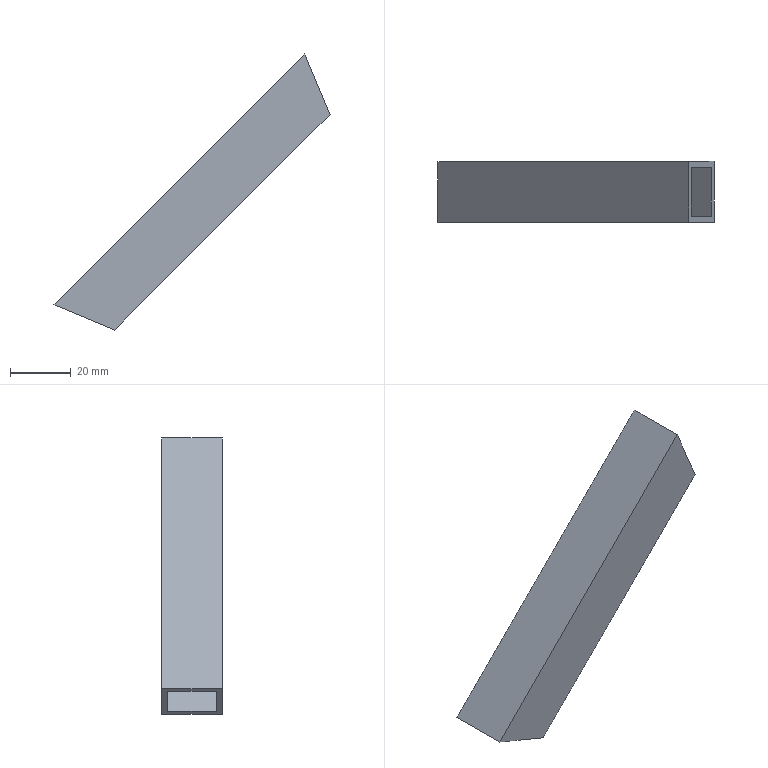Part | NX | features BREP 1 | 1 solid | 10 faces | box 90.584 x 20 x 90.584 mm | volume 15567 mm3 | plane 10
STEP:
#1=CARTESIAN_POINT('',(759.673,696.,1230.563));
#2=VERTEX_POINT('',#1);
#3=CARTESIAN_POINT('',(759.673,680.,1230.563));
#4=VERTEX_POINT('',#3);
#5=CARTESIAN_POINT('',(759.673,688.,1230.563));
#6=DIRECTION('',(0.,-1.,0.));
#7=VECTOR('',#6,1000.);
#8=LINE('',#5,#7);
#9=EDGE_CURVE('',#2,#4,#8,.T.);
#10=ORIENTED_EDGE('',*,*,#9,.T.);
#11=CARTESIAN_POINT('',(775.673,680.,1223.936));
#12=VERTEX_POINT('',#11);
#13=CARTESIAN_POINT('',(775.673,680.,1223.936));
#14=CARTESIAN_POINT('',(759.673,680.,1230.563));
#15=B_SPLINE_CURVE_WITH_KNOTS('',1,(#13,#14),.UNSPECIFIED.,.F.,.F.,(2,2),(-8.659,8.659),.UNSPECIFIED.);
#16=EDGE_CURVE('',#12,#4,#15,.T.);
#17=ORIENTED_EDGE('',*,*,#16,.F.);
#18=CARTESIAN_POINT('',(775.673,696.,1223.936));
#19=VERTEX_POINT('',#18);
#20=CARTESIAN_POINT('',(775.673,688.,1223.936));
#21=DIRECTION('',(0.,-1.,0.));
#22=VECTOR('',#21,1000.);
#23=LINE('',#20,#22);
#24=EDGE_CURVE('',#19,#12,#23,.T.);
#25=ORIENTED_EDGE('',*,*,#24,.F.);
#26=CARTESIAN_POINT('',(759.673,696.,1230.563));
#27=CARTESIAN_POINT('',(775.673,696.,1223.936));
#28=B_SPLINE_CURVE_WITH_KNOTS('',1,(#26,#27),.UNSPECIFIED.,.F.,.F.,(2,2),(-8.659,8.659),.UNSPECIFIED.);
#29=EDGE_CURVE('',#2,#19,#28,.T.);
#30=ORIENTED_EDGE('',*,*,#29,.F.);
#31=EDGE_LOOP('',(#10,#17,#25,#30));
#32=FACE_BOUND('',#31,.T.);
#33=CARTESIAN_POINT('',(757.673,698.,1231.392));
#34=VERTEX_POINT('',#33);
#35=CARTESIAN_POINT('',(777.673,698.,1223.108));
#36=VERTEX_POINT('',#35);
#37=CARTESIAN_POINT('',(757.673,698.,1231.392));
#38=CARTESIAN_POINT('',(777.673,698.,1223.108));
#39=B_SPLINE_CURVE_WITH_KNOTS('',1,(#37,#38),.UNSPECIFIED.,.F.,.F.,(2,2),(-10.824,10.824),.UNSPECIFIED.);
#40=EDGE_CURVE('',#34,#36,#39,.T.);
#41=ORIENTED_EDGE('',*,*,#40,.T.);
#42=CARTESIAN_POINT('',(777.673,678.,1223.108));
#43=VERTEX_POINT('',#42);
#44=CARTESIAN_POINT('',(777.673,688.,1223.108));
#45=DIRECTION('',(0.,-1.,0.));
#46=VECTOR('',#45,1000.);
#47=LINE('',#44,#46);
#48=EDGE_CURVE('',#36,#43,#47,.T.);
#49=ORIENTED_EDGE('',*,*,#48,.T.);
#50=CARTESIAN_POINT('',(757.673,678.,1231.392));
#51=VERTEX_POINT('',#50);
#52=CARTESIAN_POINT('',(757.673,678.,1231.392));
#53=CARTESIAN_POINT('',(777.673,678.,1223.108));
#54=B_SPLINE_CURVE_WITH_KNOTS('',1,(#52,#53),.UNSPECIFIED.,.F.,.F.,(2,2),(-10.824,10.824),.UNSPECIFIED.);
#55=EDGE_CURVE('',#51,#43,#54,.T.);
#56=ORIENTED_EDGE('',*,*,#55,.F.);
#57=CARTESIAN_POINT('',(757.673,688.,1231.392));
#58=DIRECTION('',(0.,-1.,0.));
#59=VECTOR('',#58,1000.);
#60=LINE('',#57,#59);
#61=EDGE_CURVE('',#34,#51,#60,.T.);
#62=ORIENTED_EDGE('',*,*,#61,.F.);
#63=EDGE_LOOP('',(#41,#49,#56,#62));
#64=FACE_BOUND('',#63,.T.);
#65=CARTESIAN_POINT('',(757.673,678.,1231.392));
#66=DIRECTION('',(0.3827,0.,0.9239));
#67=DIRECTION('',(0.9239,0.,-0.3827));
#68=AXIS2_PLACEMENT_3D('',#65,#66,#67);
#69=PLANE('',#68);
#70=ADVANCED_FACE('',(#32,#64),#69,.F.);
#71=ORIENTED_EDGE('',*,*,#24,.T.);
#72=CARTESIAN_POINT('',(847.429,680.,1295.692));
#73=VERTEX_POINT('',#72);
#74=CARTESIAN_POINT('',(847.429,680.,1295.692));
#75=CARTESIAN_POINT('',(823.511,680.,1271.773));
#76=CARTESIAN_POINT('',(799.592,680.,1247.855));
#77=CARTESIAN_POINT('',(775.673,680.,1223.936));
#78=B_SPLINE_CURVE_WITH_KNOTS('',3,(#74,#75,#76,#77),.UNSPECIFIED.,.F.,.F.,(4,4),(32.935,134.414),.UNSPECIFIED.);
#79=EDGE_CURVE('',#73,#12,#78,.T.);
#80=ORIENTED_EDGE('',*,*,#79,.F.);
#81=CARTESIAN_POINT('',(847.429,696.,1295.692));
#82=VERTEX_POINT('',#81);
#83=CARTESIAN_POINT('',(847.429,688.,1295.692));
#84=DIRECTION('',(0.,1.,0.));
#85=VECTOR('',#84,1000.);
#86=LINE('',#83,#85);
#87=EDGE_CURVE('',#73,#82,#86,.T.);
#88=ORIENTED_EDGE('',*,*,#87,.T.);
#89=CARTESIAN_POINT('',(775.673,696.,1223.936));
#90=CARTESIAN_POINT('',(799.592,696.,1247.855));
#91=CARTESIAN_POINT('',(823.511,696.,1271.773));
#92=CARTESIAN_POINT('',(847.429,696.,1295.692));
#93=B_SPLINE_CURVE_WITH_KNOTS('',3,(#89,#90,#91,#92),.UNSPECIFIED.,.F.,.F.,(4,4),(32.936,134.414),.UNSPECIFIED.);
#94=EDGE_CURVE('',#19,#82,#93,.T.);
#95=ORIENTED_EDGE('',*,*,#94,.F.);
#96=EDGE_LOOP('',(#71,#80,#88,#95));
#97=FACE_BOUND('',#96,.T.);
#98=CARTESIAN_POINT('',(787.74,698.,1236.002));
#99=DIRECTION('',(0.7071,0.,-0.7071));
#100=DIRECTION('',(0.7071,0.,0.7071));
#101=AXIS2_PLACEMENT_3D('',#98,#99,#100);
#102=PLANE('',#101);
#103=ADVANCED_FACE('',(#97),#102,.F.);
#104=ORIENTED_EDGE('',*,*,#29,.T.);
#105=ORIENTED_EDGE('',*,*,#94,.T.);
#106=CARTESIAN_POINT('',(840.802,696.,1311.692));
#107=VERTEX_POINT('',#106);
#108=CARTESIAN_POINT('',(844.116,696.,1303.692));
#109=DIRECTION('',(0.3827,0.,-0.9239));
#110=VECTOR('',#109,1000.);
#111=LINE('',#108,#110);
#112=EDGE_CURVE('',#107,#82,#111,.T.);
#113=ORIENTED_EDGE('',*,*,#112,.F.);
#114=CARTESIAN_POINT('',(800.238,696.,1271.128));
#115=DIRECTION('',(0.7071,0.,0.7071));
#116=VECTOR('',#115,1000.);
#117=LINE('',#114,#116);
#118=EDGE_CURVE('',#2,#107,#117,.T.);
#119=ORIENTED_EDGE('',*,*,#118,.F.);
#120=EDGE_LOOP('',(#104,#105,#113,#119));
#121=FACE_BOUND('',#120,.T.);
#122=CARTESIAN_POINT('',(805.894,696.,1265.471));
#123=DIRECTION('',(0.,1.,0.));
#124=DIRECTION('',(-1.,0.,0.));
#125=AXIS2_PLACEMENT_3D('',#122,#123,#124);
#126=PLANE('',#125);
#127=ADVANCED_FACE('',(#121),#126,.F.);
#128=ORIENTED_EDGE('',*,*,#118,.T.);
#129=CARTESIAN_POINT('',(840.802,680.,1311.692));
#130=VERTEX_POINT('',#129);
#131=CARTESIAN_POINT('',(840.802,688.,1311.692));
#132=DIRECTION('',(0.,1.,0.));
#133=VECTOR('',#132,1000.);
#134=LINE('',#131,#133);
#135=EDGE_CURVE('',#130,#107,#134,.T.);
#136=ORIENTED_EDGE('',*,*,#135,.F.);
#137=CARTESIAN_POINT('',(840.802,680.,1311.692));
#138=CARTESIAN_POINT('',(813.759,680.,1284.649));
#139=CARTESIAN_POINT('',(786.716,680.,1257.606));
#140=CARTESIAN_POINT('',(759.673,680.,1230.563));
#141=B_SPLINE_CURVE_WITH_KNOTS('',3,(#137,#138,#139,#140),.UNSPECIFIED.,.F.,.F.,(4,4),(26.308,141.041),.UNSPECIFIED.);
#142=EDGE_CURVE('',#130,#4,#141,.T.);
#143=ORIENTED_EDGE('',*,*,#142,.T.);
#144=ORIENTED_EDGE('',*,*,#9,.F.);
#145=EDGE_LOOP('',(#128,#136,#143,#144));
#146=FACE_BOUND('',#145,.T.);
#147=CARTESIAN_POINT('',(776.426,698.,1247.316));
#148=DIRECTION('',(0.7071,0.,-0.7071));
#149=DIRECTION('',(0.7071,0.,0.7071));
#150=AXIS2_PLACEMENT_3D('',#147,#148,#149);
#151=PLANE('',#150);
#152=ADVANCED_FACE('',(#146),#151,.T.);
#153=ORIENTED_EDGE('',*,*,#142,.F.);
#154=CARTESIAN_POINT('',(844.116,680.,1303.692));
#155=DIRECTION('',(-0.3827,0.,0.9239));
#156=VECTOR('',#155,1000.);
#157=LINE('',#154,#156);
#158=EDGE_CURVE('',#73,#130,#157,.T.);
#159=ORIENTED_EDGE('',*,*,#158,.F.);
#160=ORIENTED_EDGE('',*,*,#79,.T.);
#161=ORIENTED_EDGE('',*,*,#16,.T.);
#162=EDGE_LOOP('',(#153,#159,#160,#161));
#163=FACE_BOUND('',#162,.T.);
#164=CARTESIAN_POINT('',(805.894,680.,1265.471));
#165=DIRECTION('',(0.,1.,0.));
#166=DIRECTION('',(0.,0.,1.));
#167=AXIS2_PLACEMENT_3D('',#164,#165,#166);
#168=PLANE('',#167);
#169=ADVANCED_FACE('',(#163),#168,.T.);
#170=CARTESIAN_POINT('',(839.974,698.,1313.692));
#171=VERTEX_POINT('',#170);
#172=CARTESIAN_POINT('',(798.823,698.,1272.542));
#173=DIRECTION('',(0.7071,0.,0.7071));
#174=VECTOR('',#173,1000.);
#175=LINE('',#172,#174);
#176=EDGE_CURVE('',#34,#171,#175,.T.);
#177=ORIENTED_EDGE('',*,*,#176,.T.);
#178=CARTESIAN_POINT('',(848.258,698.,1293.692));
#179=VERTEX_POINT('',#178);
#180=CARTESIAN_POINT('',(844.116,698.,1303.692));
#181=DIRECTION('',(0.3827,0.,-0.9239));
#182=VECTOR('',#181,1000.);
#183=LINE('',#180,#182);
#184=EDGE_CURVE('',#171,#179,#183,.T.);
#185=ORIENTED_EDGE('',*,*,#184,.T.);
#186=CARTESIAN_POINT('',(812.966,698.,1258.4));
#187=DIRECTION('',(0.7071,0.,0.7071));
#188=VECTOR('',#187,1000.);
#189=LINE('',#186,#188);
#190=EDGE_CURVE('',#36,#179,#189,.T.);
#191=ORIENTED_EDGE('',*,*,#190,.F.);
#192=ORIENTED_EDGE('',*,*,#40,.F.);
#193=EDGE_LOOP('',(#177,#185,#191,#192));
#194=FACE_BOUND('',#193,.T.);
#195=CARTESIAN_POINT('',(805.894,698.,1265.471));
#196=DIRECTION('',(0.,1.,0.));
#197=DIRECTION('',(-1.,0.,0.));
#198=AXIS2_PLACEMENT_3D('',#195,#196,#197);
#199=PLANE('',#198);
#200=ADVANCED_FACE('',(#194),#199,.T.);
#201=ORIENTED_EDGE('',*,*,#190,.T.);
#202=CARTESIAN_POINT('',(848.258,678.,1293.692));
#203=VERTEX_POINT('',#202);
#204=CARTESIAN_POINT('',(848.258,688.,1293.692));
#205=DIRECTION('',(0.,-1.,0.));
#206=VECTOR('',#205,1000.);
#207=LINE('',#204,#206);
#208=EDGE_CURVE('',#179,#203,#207,.T.);
#209=ORIENTED_EDGE('',*,*,#208,.T.);
#210=CARTESIAN_POINT('',(848.258,678.,1293.692));
#211=CARTESIAN_POINT('',(834.141,678.,1279.575));
#212=CARTESIAN_POINT('',(820.024,678.,1265.458));
#213=CARTESIAN_POINT('',(805.907,678.,1251.341));
#214=CARTESIAN_POINT('',(791.79,678.,1237.224));
#215=CARTESIAN_POINT('',(777.673,678.,1223.108));
#216=B_SPLINE_CURVE_WITH_KNOTS('',5,(#210,#211,#212,#213,#214,#215),.UNSPECIFIED.,.F.,.F.,(6,6),(33.764,133.585),.UNSPECIFIED.);
#217=EDGE_CURVE('',#203,#43,#216,.T.);
#218=ORIENTED_EDGE('',*,*,#217,.T.);
#219=ORIENTED_EDGE('',*,*,#48,.F.);
#220=EDGE_LOOP('',(#201,#209,#218,#219));
#221=FACE_BOUND('',#220,.T.);
#222=CARTESIAN_POINT('',(789.154,698.,1234.588));
#223=DIRECTION('',(0.7071,0.,-0.7071));
#224=DIRECTION('',(0.7071,0.,0.7071));
#225=AXIS2_PLACEMENT_3D('',#222,#223,#224);
#226=PLANE('',#225);
#227=ADVANCED_FACE('',(#221),#226,.T.);
#228=ORIENTED_EDGE('',*,*,#55,.T.);
#229=ORIENTED_EDGE('',*,*,#217,.F.);
#230=CARTESIAN_POINT('',(839.974,678.,1313.692));
#231=VERTEX_POINT('',#230);
#232=CARTESIAN_POINT('',(844.116,678.,1303.692));
#233=DIRECTION('',(0.3827,0.,-0.9239));
#234=VECTOR('',#233,1000.);
#235=LINE('',#232,#234);
#236=EDGE_CURVE('',#231,#203,#235,.T.);
#237=ORIENTED_EDGE('',*,*,#236,.F.);
#238=CARTESIAN_POINT('',(798.823,678.,1272.542));
#239=DIRECTION('',(0.7071,0.,0.7071));
#240=VECTOR('',#239,1000.);
#241=LINE('',#238,#240);
#242=EDGE_CURVE('',#51,#231,#241,.T.);
#243=ORIENTED_EDGE('',*,*,#242,.F.);
#244=EDGE_LOOP('',(#228,#229,#237,#243));
#245=FACE_BOUND('',#244,.T.);
#246=CARTESIAN_POINT('',(805.894,678.,1265.471));
#247=DIRECTION('',(0.,1.,0.));
#248=DIRECTION('',(0.,0.,1.));
#249=AXIS2_PLACEMENT_3D('',#246,#247,#248);
#250=PLANE('',#249);
#251=ADVANCED_FACE('',(#245),#250,.F.);
#252=ORIENTED_EDGE('',*,*,#61,.T.);
#253=ORIENTED_EDGE('',*,*,#242,.T.);
#254=CARTESIAN_POINT('',(839.974,688.,1313.692));
#255=DIRECTION('',(0.,1.,0.));
#256=VECTOR('',#255,1000.);
#257=LINE('',#254,#256);
#258=EDGE_CURVE('',#231,#171,#257,.T.);
#259=ORIENTED_EDGE('',*,*,#258,.T.);
#260=ORIENTED_EDGE('',*,*,#176,.F.);
#261=EDGE_LOOP('',(#252,#253,#259,#260));
#262=FACE_BOUND('',#261,.T.);
#263=CARTESIAN_POINT('',(775.012,698.,1248.73));
#264=DIRECTION('',(0.7071,0.,-0.7071));
#265=DIRECTION('',(0.7071,0.,0.7071));
#266=AXIS2_PLACEMENT_3D('',#263,#264,#265);
#267=PLANE('',#266);
#268=ADVANCED_FACE('',(#262),#267,.F.);
#269=ORIENTED_EDGE('',*,*,#158,.T.);
#270=ORIENTED_EDGE('',*,*,#135,.T.);
#271=ORIENTED_EDGE('',*,*,#112,.T.);
#272=ORIENTED_EDGE('',*,*,#87,.F.);
#273=EDGE_LOOP('',(#269,#270,#271,#272));
#274=FACE_BOUND('',#273,.T.);
#275=ORIENTED_EDGE('',*,*,#258,.F.);
#276=ORIENTED_EDGE('',*,*,#236,.T.);
#277=ORIENTED_EDGE('',*,*,#208,.F.);
#278=ORIENTED_EDGE('',*,*,#184,.F.);
#279=EDGE_LOOP('',(#275,#276,#277,#278));
#280=FACE_BOUND('',#279,.T.);
#281=CARTESIAN_POINT('',(839.974,678.,1313.692));
#282=DIRECTION('',(0.9239,0.,0.3827));
#283=DIRECTION('',(0.3827,0.,-0.9239));
#284=AXIS2_PLACEMENT_3D('',#281,#282,#283);
#285=PLANE('',#284);
#286=ADVANCED_FACE('',(#274,#280),#285,.T.);
#287=CLOSED_SHELL('',(#70,#103,#127,#152,#169,#200,#227,#251,#268,#286));
#288=MANIFOLD_SOLID_BREP('',#287);
#289=(LENGTH_UNIT()NAMED_UNIT(*)SI_UNIT(.MILLI.,.METRE.));
#290=UNCERTAINTY_MEASURE_WITH_UNIT(LENGTH_MEASURE(0.00001),#289,'','');
#291=(NAMED_UNIT(*)PLANE_ANGLE_UNIT()SI_UNIT($,.RADIAN.));
#292=(NAMED_UNIT(*)SI_UNIT($,.STERADIAN.)SOLID_ANGLE_UNIT());
#293=(GEOMETRIC_REPRESENTATION_CONTEXT(3)GLOBAL_UNCERTAINTY_ASSIGNED_CONTEXT((#290))GLOBAL_UNIT_ASSIGNED_CONTEXT((#289,#291,#292))REPRESENTATION_CONTEXT('',''));
#294=ADVANCED_BREP_SHAPE_REPRESENTATION('',(#288),#293);